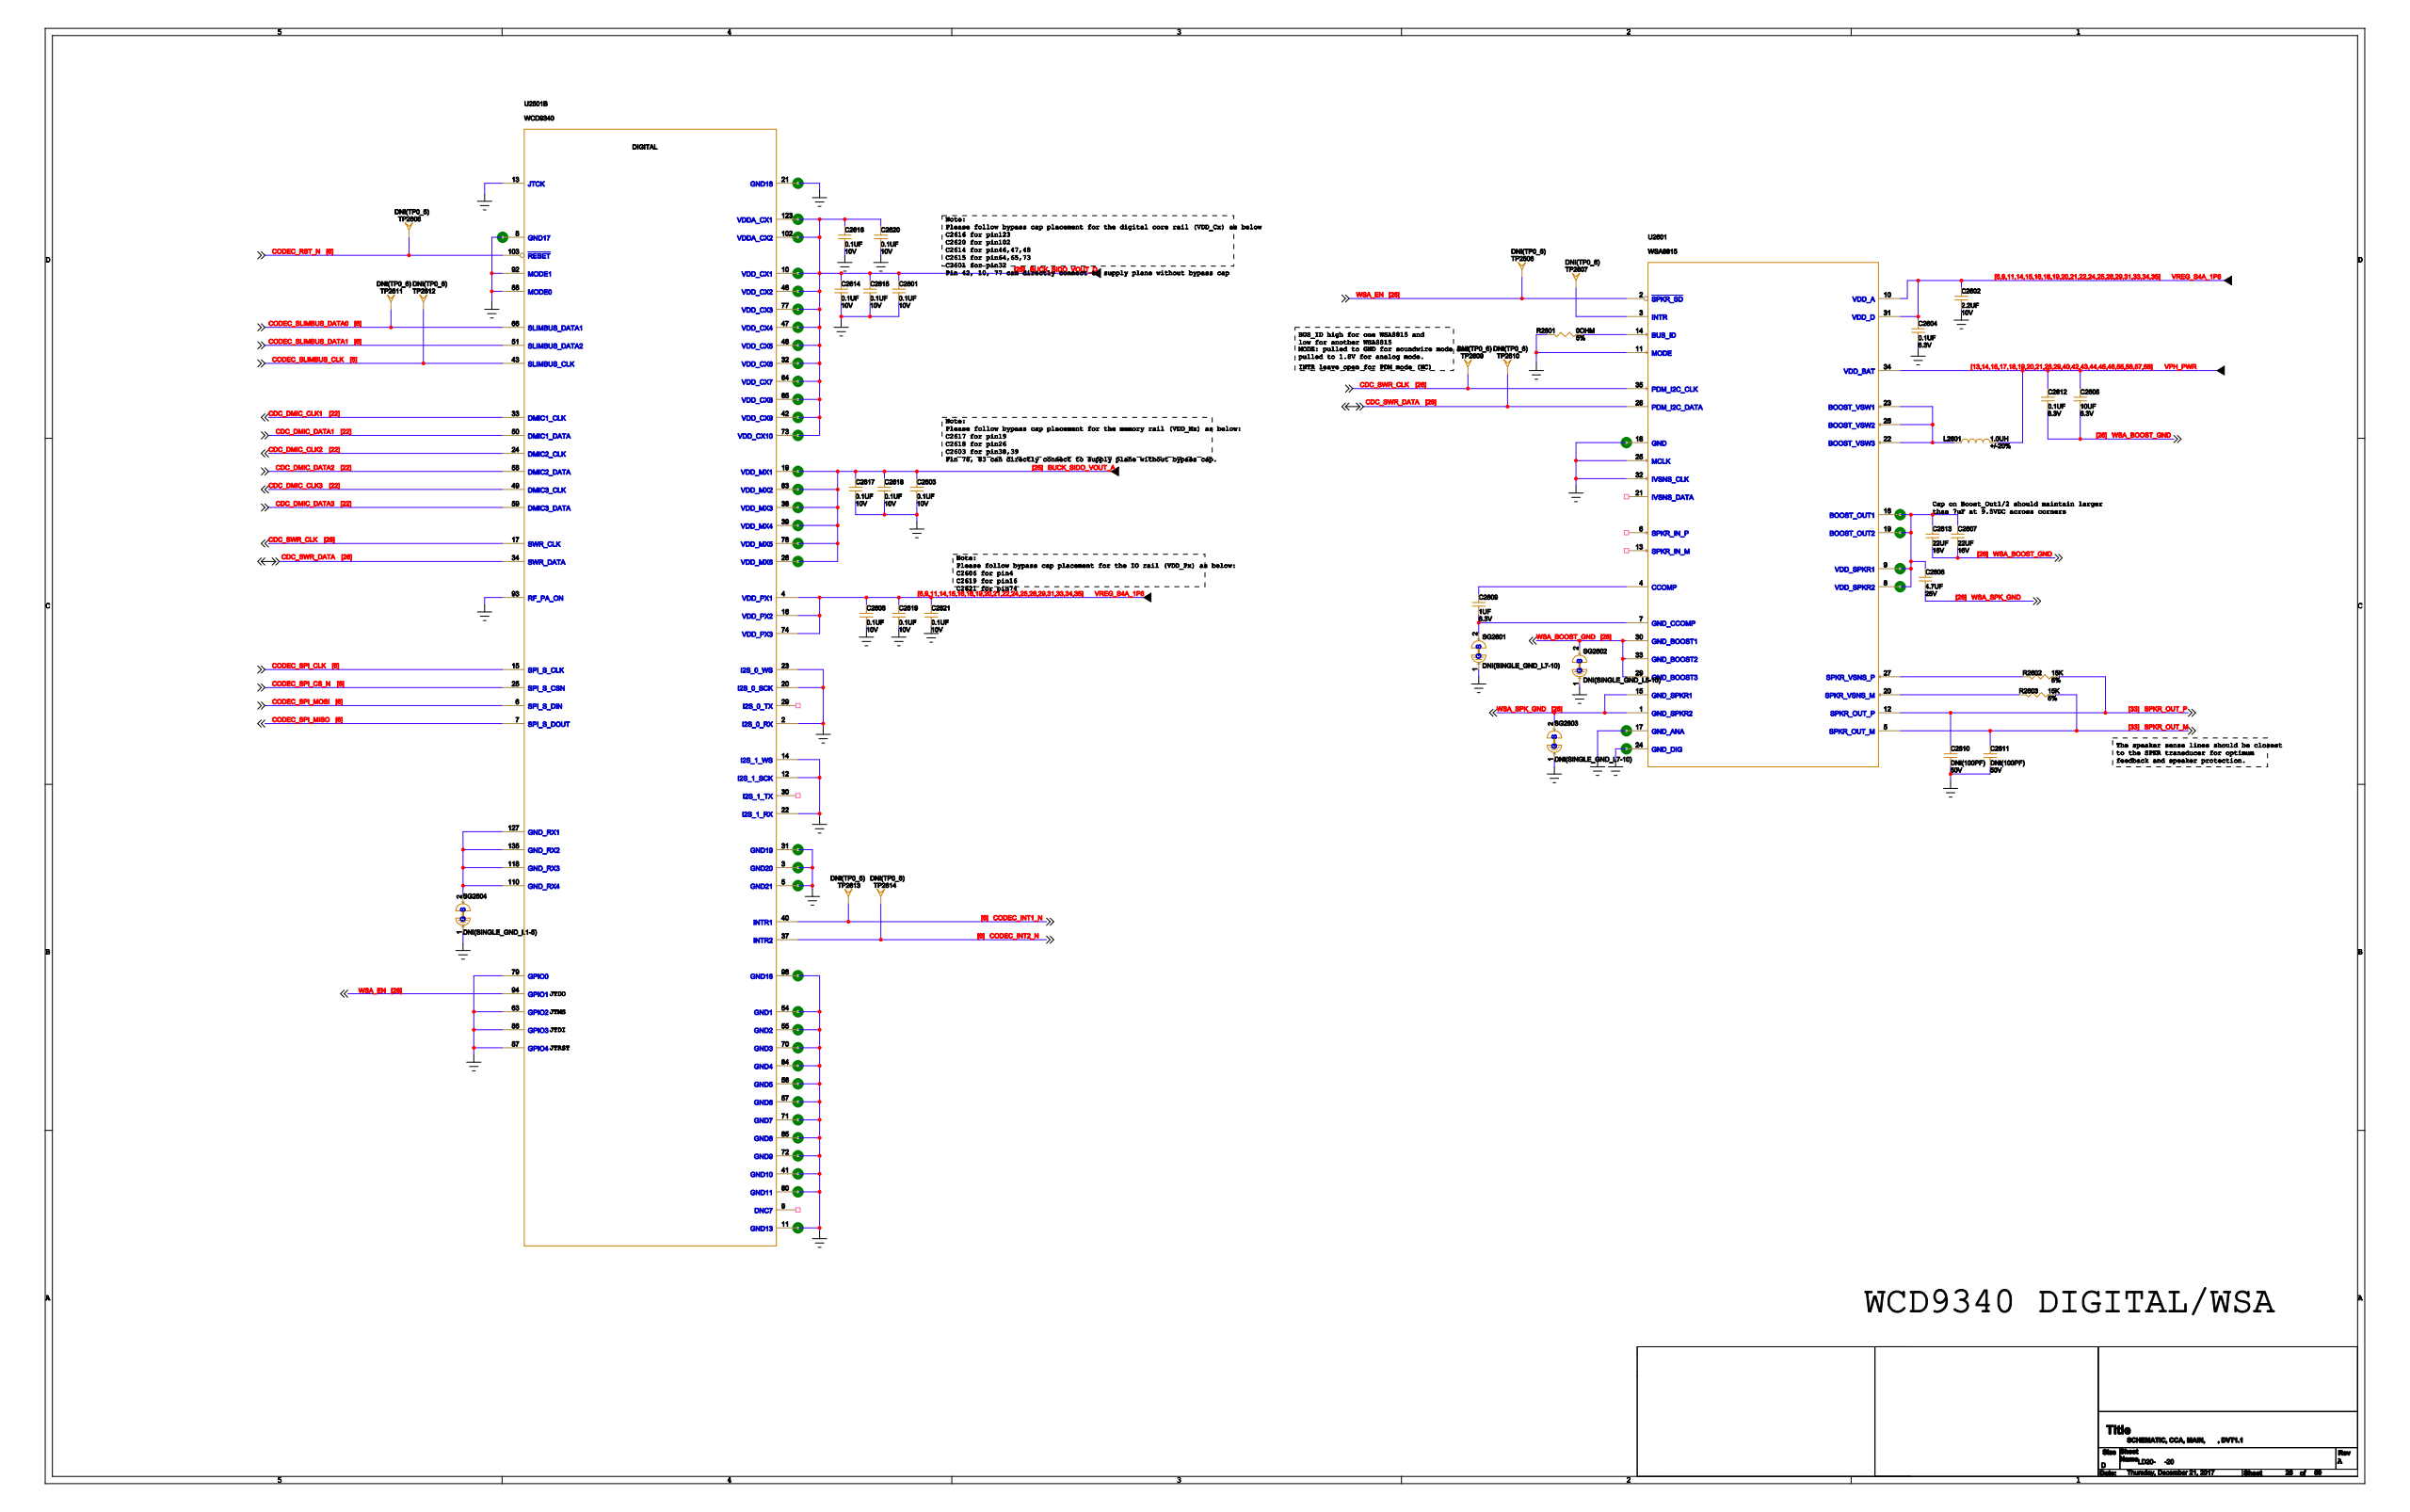Circuit board | Cadence Allegro | 1520 parts | 1149 nets | one sheet of the schematic
Parts on this sheet (reference | value | footprint):
C2601 | 0.1UF | 2P0201R
C2602 | 2.2UF | 2P0201R
C2603 | 0.1UF | 2P0201R
C2604 | 0.1UF | 2P0201R
C2605 | 10UF | 2P0603R
C2606 | 0.1UF | 2P0201R
C2607 | 22UF | 2P0805R
C2608 | 4.7UF | 2P0603R
C2609 | 1UF | 2P0201R
C2610 | DNI(100PF) | 2P0201R_DNI
C2611 | DNI(100PF) | 2P0201R_DNI
C2612 | 0.1UF | 2P0201R
C2613 | 22UF | 2P0805R
C2614 | 0.1UF | 2P0201R
C2615 | 0.1UF | 2P0201R
C2616 | 0.1UF | 2P0201R
C2617 | 0.1UF | 2P0201R
C2618 | 0.1UF | 2P0201R
C2619 | 0.1UF | 2P0201R
C2620 | 0.1UF | 2P0201R
C2621 | 0.1UF | 2P0201R
L2601 | 1.0UH | 2PSM87X71NV2
R2601 | 0OHM | 2P0201R
R2602 | 15K | 2P0201R
R2603 | 15K | 2P0201R
SG2601 | DNI(SINGLE_GND_L7-10) | GND_L7-10
SG2602 | DNI(SINGLE_GND_L5-10) | GND_L5-10
SG2603 | DNI(SINGLE_GND_L7-10) | GND_L7-10
SG2604 | DNI(SINGLE_GND_L1-5) | GND_L1-5
TP2606 | DNI(TP0_6) | TP-0_6
TP2607 | DNI(TP0_6) | TP-0_6
TP2608 | DNI(TP0_6) | TP-0_6
TP2609 | DNI(TP0_6) | TP-0_6
TP2610 | DNI(TP0_6) | TP-0_6
TP2611 | DNI(TP0_6) | TP-0_6
TP2612 | DNI(TP0_6) | TP-0_6
TP2613 | DNI(TP0_6) | TP-0_6
TP2614 | DNI(TP0_6) | TP-0_6
U2501 | WCD9340 | 154PGA196X171B138D45
U2601 | WSA8815 | 35PGA90X105B157D60
Nets of these parts (net: part-pin ...):
GND: C2601-2 C2602-2 C2603-2 C2604-2 C2606-2 C2610-2 C2611-2 C2614-2 C2615-2 C2616-2 C2617-2 C2618-2 C2619-2 C2620-2 C2621-2 R2601-1 SG2601-1 SG2602-1 SG2603-1 SG2604-1 U2501-2 U2501-3 U2501-5 U2501-8 U2501-11 U2501-12 U2501-13 U2501-14 U2501-18 U2501-20 U2501-21 U2501-22 U2501-23 U2501-31 U2501-41 U2501-54 U2501-55 U2501-56 U2501-57 U2501-63 U2501-70 U2501-71 U2501-72 U2501-79 U2501-80 U2501-84 U2501-85 U2501-86 U2501-87 U2501-88 U2501-92 U2501-93 U2501-98 U2601-11 U2601-17 U2601-18 U2601-24 U2601-25 U2601-32
VREG_S4A_1P8: C2602-1 C2604-1 C2606-1 C2619-1 C2621-1 U2501-4 U2501-16 U2501-74 U2601-10 U2601-31
N36384548: SG2604-2 U2501-110 U2501-118 U2501-127 U2501-135
WSA_BOOST_GND: C2605-2 C2607-2 C2612-2 C2613-2 SG2602-2 U2601-29 U2601-30 U2601-33
N32078893: C2609-2 SG2601-2 U2601-7
WSA_SPK_GND: C2608-2 SG2603-2 U2601-1 U2601-15
VPH_PWR: C2605-1 C2612-1 L2601-2 U2601-34
CDC_DMIC_DATA3: U2501-59
CDC_DMIC_CLK3: U2501-49
CDC_DMIC_CLK1: U2501-33
CDC_DMIC_DATA1: U2501-50
CDC_DMIC_CLK2: U2501-24
CDC_DMIC_DATA2: U2501-58
BUCK_SIDO_VOUT_A: C2603-1 C2617-1 C2618-1 U2501-19 U2501-26 U2501-38 U2501-39 U2501-78 U2501-83
BUCK_SIDO_VOUT_D: C2601-1 C2614-1 C2615-1 C2616-1 C2620-1 U2501-10 U2501-32 U2501-42 U2501-46 U2501-47 U2501-48 U2501-64 U2501-65 U2501-73 U2501-77 U2501-102 U2501-123
WSA_EN: TP2606-1 U2501-94 U2601-2
CODEC_INT1_N: TP2613-1 U2501-40
CODEC_INT2_N: TP2614-1 U2501-37
CODEC_RST_N: TP2608-1 U2501-103
CODEC_SLIMBUS_CLK: TP2612-1 U2501-43
CODEC_SLIMBUS_DATA0: TP2611-1 U2501-66
CODEC_SLIMBUS_DATA1: U2501-51
CODEC_SPI_CLK: U2501-15
CODEC_SPI_CS_N: U2501-25
CODEC_SPI_MOSI: U2501-6
CODEC_SPI_MISO: U2501-7
CDC_SWR_CLK: TP2609-1 U2501-17 U2601-35
CDC_SWR_DATA: TP2610-1 U2501-34 U2601-28
N32018899: C2609-1 U2601-4
SPKR_OUT_M: C2611-1 R2603-2 U2601-5
SPKR_OUT_P: C2610-1 R2602-2 U2601-12
N32017443: C2607-1 C2608-1 C2613-1 U2601-8 U2601-9 U2601-16 U2601-19
N32033941: R2601-2 U2601-14
N32017004: L2601-1 U2601-22 U2601-23 U2601-26
N32018192: R2602-1 U2601-27
N32018430: R2603-1 U2601-20
N32020358: TP2607-1 U2601-3